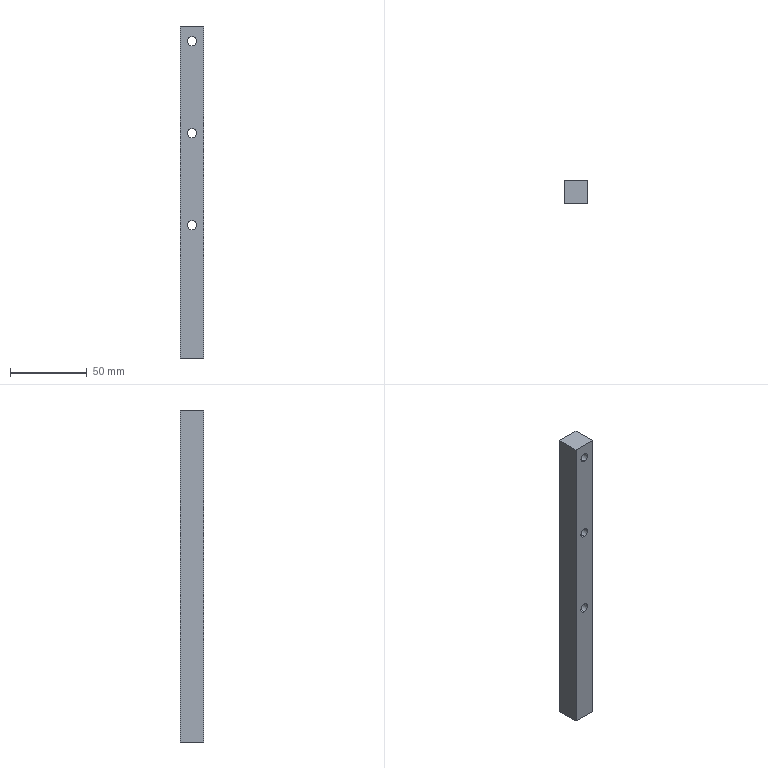Part | 1 solid | 16 faces | box 15 x 15 x 216.5 mm | volume 46834 mm3 | cylinder 8 | plane 6 | cone 2 | commonest cylinder face diameters 6 x6 6.8 x2
STEP:
#1=CARTESIAN_POINT('',(10.9,7.5,59.5));
#2=VERTEX_POINT('',#1);
#3=CARTESIAN_POINT('',(4.1,7.5,59.5));
#4=VERTEX_POINT('',#3);
#5=CARTESIAN_POINT('',(7.5,7.5,59.5));
#6=DIRECTION('',(0.,0.,-1.));
#7=DIRECTION('',(-1.,0.,0.));
#8=AXIS2_PLACEMENT_3D('',#5,#6,#7);
#9=CIRCLE('',#8,3.4);
#10=EDGE_CURVE('',#2,#4,#9,.T.);
#11=ORIENTED_EDGE('',*,*,#10,.F.);
#12=CARTESIAN_POINT('',(10.9,7.5,43.5));
#13=VERTEX_POINT('',#12);
#14=CARTESIAN_POINT('',(10.9,7.5,43.5));
#15=DIRECTION('',(0.,0.,-1.));
#16=VECTOR('',#15,1000.);
#17=LINE('',#14,#16);
#18=EDGE_CURVE('',#2,#13,#17,.T.);
#19=ORIENTED_EDGE('',*,*,#18,.T.);
#20=CARTESIAN_POINT('',(4.1,7.5,43.5));
#21=VERTEX_POINT('',#20);
#22=CARTESIAN_POINT('',(7.5,7.5,43.5));
#23=DIRECTION('',(0.,0.,-1.));
#24=DIRECTION('',(-1.,0.,0.));
#25=AXIS2_PLACEMENT_3D('',#22,#23,#24);
#26=CIRCLE('',#25,3.4);
#27=EDGE_CURVE('',#13,#21,#26,.T.);
#28=ORIENTED_EDGE('',*,*,#27,.T.);
#29=CARTESIAN_POINT('',(4.1,7.5,43.5));
#30=DIRECTION('',(0.,0.,-1.));
#31=VECTOR('',#30,1000.);
#32=LINE('',#29,#31);
#33=EDGE_CURVE('',#4,#21,#32,.T.);
#34=ORIENTED_EDGE('',*,*,#33,.F.);
#35=EDGE_LOOP('',(#11,#19,#28,#34));
#36=FACE_OUTER_BOUND('',#35,.T.);
#37=CARTESIAN_POINT('',(7.5,7.5,43.5));
#38=DIRECTION('',(0.,0.,-1.));
#39=DIRECTION('',(-1.,0.,0.));
#40=AXIS2_PLACEMENT_3D('',#37,#38,#39);
#41=CYLINDRICAL_SURFACE('',#40,3.4);
#42=ADVANCED_FACE('',(#36),#41,.F.);
#43=CARTESIAN_POINT('',(7.5,7.5,61.543));
#44=VERTEX_POINT('',#43);
#45=CARTESIAN_POINT('',(4.1,7.5,59.5));
#46=DIRECTION('',(-0.8572,0.,-0.515));
#47=VECTOR('',#46,1000.);
#48=LINE('',#45,#47);
#49=EDGE_CURVE('',#44,#4,#48,.T.);
#50=ORIENTED_EDGE('',*,*,#49,.F.);
#51=CARTESIAN_POINT('',(10.9,7.5,59.5));
#52=DIRECTION('',(0.8572,0.,-0.515));
#53=VECTOR('',#52,1000.);
#54=LINE('',#51,#53);
#55=EDGE_CURVE('',#44,#2,#54,.T.);
#56=ORIENTED_EDGE('',*,*,#55,.T.);
#57=ORIENTED_EDGE('',*,*,#10,.T.);
#58=EDGE_LOOP('',(#50,#56,#57));
#59=FACE_OUTER_BOUND('',#58,.T.);
#60=CARTESIAN_POINT('',(7.5,7.5,59.5));
#61=DIRECTION('',(0.,0.,-1.));
#62=DIRECTION('',(-1.,0.,0.));
#63=AXIS2_PLACEMENT_3D('',#60,#61,#62);
#64=CONICAL_SURFACE('',#63,3.4,1.03);
#65=ADVANCED_FACE('',(#59),#64,.F.);
#66=CARTESIAN_POINT('',(7.5,0.,247.));
#67=VERTEX_POINT('',#66);
#68=CARTESIAN_POINT('',(7.5,0.,253.));
#69=VERTEX_POINT('',#68);
#70=CARTESIAN_POINT('',(7.5,0.,250.));
#71=DIRECTION('',(0.,1.,0.));
#72=DIRECTION('',(0.,0.,1.));
#73=AXIS2_PLACEMENT_3D('',#70,#71,#72);
#74=CIRCLE('',#73,3.);
#75=EDGE_CURVE('',#67,#69,#74,.T.);
#76=ORIENTED_EDGE('',*,*,#75,.F.);
#77=CARTESIAN_POINT('',(7.5,15.,247.));
#78=VERTEX_POINT('',#77);
#79=CARTESIAN_POINT('',(7.5,-35.,247.));
#80=DIRECTION('',(0.,1.,0.));
#81=VECTOR('',#80,1000.);
#82=LINE('',#79,#81);
#83=EDGE_CURVE('',#67,#78,#82,.T.);
#84=ORIENTED_EDGE('',*,*,#83,.T.);
#85=CARTESIAN_POINT('',(7.5,15.,253.));
#86=VERTEX_POINT('',#85);
#87=CARTESIAN_POINT('',(7.5,15.,250.));
#88=DIRECTION('',(0.,1.,0.));
#89=DIRECTION('',(0.,0.,1.));
#90=AXIS2_PLACEMENT_3D('',#87,#88,#89);
#91=CIRCLE('',#90,3.);
#92=EDGE_CURVE('',#78,#86,#91,.T.);
#93=ORIENTED_EDGE('',*,*,#92,.T.);
#94=CARTESIAN_POINT('',(7.5,-35.,253.));
#95=DIRECTION('',(0.,1.,0.));
#96=VECTOR('',#95,1000.);
#97=LINE('',#94,#96);
#98=EDGE_CURVE('',#69,#86,#97,.T.);
#99=ORIENTED_EDGE('',*,*,#98,.F.);
#100=EDGE_LOOP('',(#76,#84,#93,#99));
#101=FACE_OUTER_BOUND('',#100,.T.);
#102=CARTESIAN_POINT('',(7.5,-35.,250.));
#103=DIRECTION('',(0.,1.,0.));
#104=DIRECTION('',(0.,0.,1.));
#105=AXIS2_PLACEMENT_3D('',#102,#103,#104);
#106=CYLINDRICAL_SURFACE('',#105,3.);
#107=ADVANCED_FACE('',(#101),#106,.F.);
#108=CARTESIAN_POINT('',(7.5,0.,187.));
#109=VERTEX_POINT('',#108);
#110=CARTESIAN_POINT('',(7.5,0.,193.));
#111=VERTEX_POINT('',#110);
#112=CARTESIAN_POINT('',(7.5,0.,190.));
#113=DIRECTION('',(0.,1.,0.));
#114=DIRECTION('',(0.,0.,1.));
#115=AXIS2_PLACEMENT_3D('',#112,#113,#114);
#116=CIRCLE('',#115,3.);
#117=EDGE_CURVE('',#109,#111,#116,.T.);
#118=ORIENTED_EDGE('',*,*,#117,.F.);
#119=CARTESIAN_POINT('',(7.5,15.,187.));
#120=VERTEX_POINT('',#119);
#121=CARTESIAN_POINT('',(7.5,-35.,187.));
#122=DIRECTION('',(0.,1.,0.));
#123=VECTOR('',#122,1000.);
#124=LINE('',#121,#123);
#125=EDGE_CURVE('',#109,#120,#124,.T.);
#126=ORIENTED_EDGE('',*,*,#125,.T.);
#127=CARTESIAN_POINT('',(7.5,15.,193.));
#128=VERTEX_POINT('',#127);
#129=CARTESIAN_POINT('',(7.5,15.,190.));
#130=DIRECTION('',(0.,1.,0.));
#131=DIRECTION('',(0.,0.,1.));
#132=AXIS2_PLACEMENT_3D('',#129,#130,#131);
#133=CIRCLE('',#132,3.);
#134=EDGE_CURVE('',#120,#128,#133,.T.);
#135=ORIENTED_EDGE('',*,*,#134,.T.);
#136=CARTESIAN_POINT('',(7.5,-35.,193.));
#137=DIRECTION('',(0.,1.,0.));
#138=VECTOR('',#137,1000.);
#139=LINE('',#136,#138);
#140=EDGE_CURVE('',#111,#128,#139,.T.);
#141=ORIENTED_EDGE('',*,*,#140,.F.);
#142=EDGE_LOOP('',(#118,#126,#135,#141));
#143=FACE_OUTER_BOUND('',#142,.T.);
#144=CARTESIAN_POINT('',(7.5,-35.,190.));
#145=DIRECTION('',(0.,1.,0.));
#146=DIRECTION('',(0.,0.,1.));
#147=AXIS2_PLACEMENT_3D('',#144,#145,#146);
#148=CYLINDRICAL_SURFACE('',#147,3.);
#149=ADVANCED_FACE('',(#143),#148,.F.);
#150=CARTESIAN_POINT('',(7.5,0.,127.));
#151=VERTEX_POINT('',#150);
#152=CARTESIAN_POINT('',(7.5,0.,133.));
#153=VERTEX_POINT('',#152);
#154=CARTESIAN_POINT('',(7.5,0.,130.));
#155=DIRECTION('',(0.,1.,0.));
#156=DIRECTION('',(0.,0.,1.));
#157=AXIS2_PLACEMENT_3D('',#154,#155,#156);
#158=CIRCLE('',#157,3.);
#159=EDGE_CURVE('',#151,#153,#158,.T.);
#160=ORIENTED_EDGE('',*,*,#159,.F.);
#161=CARTESIAN_POINT('',(7.5,15.,127.));
#162=VERTEX_POINT('',#161);
#163=CARTESIAN_POINT('',(7.5,-35.,127.));
#164=DIRECTION('',(0.,1.,0.));
#165=VECTOR('',#164,1000.);
#166=LINE('',#163,#165);
#167=EDGE_CURVE('',#151,#162,#166,.T.);
#168=ORIENTED_EDGE('',*,*,#167,.T.);
#169=CARTESIAN_POINT('',(7.5,15.,133.));
#170=VERTEX_POINT('',#169);
#171=CARTESIAN_POINT('',(7.5,15.,130.));
#172=DIRECTION('',(0.,1.,0.));
#173=DIRECTION('',(0.,0.,1.));
#174=AXIS2_PLACEMENT_3D('',#171,#172,#173);
#175=CIRCLE('',#174,3.);
#176=EDGE_CURVE('',#162,#170,#175,.T.);
#177=ORIENTED_EDGE('',*,*,#176,.T.);
#178=CARTESIAN_POINT('',(7.5,-35.,133.));
#179=DIRECTION('',(0.,1.,0.));
#180=VECTOR('',#179,1000.);
#181=LINE('',#178,#180);
#182=EDGE_CURVE('',#153,#170,#181,.T.);
#183=ORIENTED_EDGE('',*,*,#182,.F.);
#184=EDGE_LOOP('',(#160,#168,#177,#183));
#185=FACE_OUTER_BOUND('',#184,.T.);
#186=CARTESIAN_POINT('',(7.5,-35.,130.));
#187=DIRECTION('',(0.,1.,0.));
#188=DIRECTION('',(0.,0.,1.));
#189=AXIS2_PLACEMENT_3D('',#186,#187,#188);
#190=CYLINDRICAL_SURFACE('',#189,3.);
#191=ADVANCED_FACE('',(#185),#190,.F.);
#192=CARTESIAN_POINT('',(0.,15.,260.));
#193=VERTEX_POINT('',#192);
#194=CARTESIAN_POINT('',(0.,15.,43.5));
#195=VERTEX_POINT('',#194);
#196=CARTESIAN_POINT('',(0.,15.,700.));
#197=DIRECTION('',(0.,0.,-1.));
#198=VECTOR('',#197,1000.);
#199=LINE('',#196,#198);
#200=EDGE_CURVE('',#193,#195,#199,.T.);
#201=ORIENTED_EDGE('',*,*,#200,.T.);
#202=CARTESIAN_POINT('',(0.,0.,43.5));
#203=VERTEX_POINT('',#202);
#204=CARTESIAN_POINT('',(0.,15.,43.5));
#205=DIRECTION('',(0.,1.,0.));
#206=VECTOR('',#205,1000.);
#207=LINE('',#204,#206);
#208=EDGE_CURVE('',#203,#195,#207,.T.);
#209=ORIENTED_EDGE('',*,*,#208,.F.);
#210=CARTESIAN_POINT('',(0.,0.,260.));
#211=VERTEX_POINT('',#210);
#212=CARTESIAN_POINT('',(0.,0.,700.));
#213=DIRECTION('',(0.,0.,-1.));
#214=VECTOR('',#213,1000.);
#215=LINE('',#212,#214);
#216=EDGE_CURVE('',#211,#203,#215,.T.);
#217=ORIENTED_EDGE('',*,*,#216,.F.);
#218=CARTESIAN_POINT('',(0.,15.,260.));
#219=DIRECTION('',(0.,-1.,0.));
#220=VECTOR('',#219,1000.);
#221=LINE('',#218,#220);
#222=EDGE_CURVE('',#193,#211,#221,.T.);
#223=ORIENTED_EDGE('',*,*,#222,.F.);
#224=EDGE_LOOP('',(#201,#209,#217,#223));
#225=FACE_OUTER_BOUND('',#224,.T.);
#226=CARTESIAN_POINT('',(0.,0.,700.));
#227=DIRECTION('',(1.,0.,0.));
#228=DIRECTION('',(0.,0.,-1.));
#229=AXIS2_PLACEMENT_3D('',#226,#227,#228);
#230=PLANE('',#229);
#231=ADVANCED_FACE('',(#225),#230,.F.);
#232=CARTESIAN_POINT('',(7.5,0.,130.));
#233=DIRECTION('',(0.,1.,0.));
#234=DIRECTION('',(0.,0.,1.));
#235=AXIS2_PLACEMENT_3D('',#232,#233,#234);
#236=CIRCLE('',#235,3.);
#237=EDGE_CURVE('',#153,#151,#236,.T.);
#238=ORIENTED_EDGE('',*,*,#237,.T.);
#239=ORIENTED_EDGE('',*,*,#159,.T.);
#240=EDGE_LOOP('',(#238,#239));
#241=FACE_BOUND('',#240,.T.);
#242=CARTESIAN_POINT('',(7.5,0.,190.));
#243=DIRECTION('',(0.,1.,0.));
#244=DIRECTION('',(0.,0.,1.));
#245=AXIS2_PLACEMENT_3D('',#242,#243,#244);
#246=CIRCLE('',#245,3.);
#247=EDGE_CURVE('',#111,#109,#246,.T.);
#248=ORIENTED_EDGE('',*,*,#247,.T.);
#249=ORIENTED_EDGE('',*,*,#117,.T.);
#250=EDGE_LOOP('',(#248,#249));
#251=FACE_BOUND('',#250,.T.);
#252=CARTESIAN_POINT('',(7.5,0.,250.));
#253=DIRECTION('',(0.,1.,0.));
#254=DIRECTION('',(0.,0.,1.));
#255=AXIS2_PLACEMENT_3D('',#252,#253,#254);
#256=CIRCLE('',#255,3.);
#257=EDGE_CURVE('',#69,#67,#256,.T.);
#258=ORIENTED_EDGE('',*,*,#257,.T.);
#259=ORIENTED_EDGE('',*,*,#75,.T.);
#260=EDGE_LOOP('',(#258,#259));
#261=FACE_BOUND('',#260,.T.);
#262=ORIENTED_EDGE('',*,*,#216,.T.);
#263=CARTESIAN_POINT('',(15.,0.,43.5));
#264=VERTEX_POINT('',#263);
#265=CARTESIAN_POINT('',(15.,0.,43.5));
#266=DIRECTION('',(-1.,0.,0.));
#267=VECTOR('',#266,1000.);
#268=LINE('',#265,#267);
#269=EDGE_CURVE('',#264,#203,#268,.T.);
#270=ORIENTED_EDGE('',*,*,#269,.F.);
#271=CARTESIAN_POINT('',(15.,0.,260.));
#272=VERTEX_POINT('',#271);
#273=CARTESIAN_POINT('',(15.,0.,700.));
#274=DIRECTION('',(0.,0.,-1.));
#275=VECTOR('',#274,1000.);
#276=LINE('',#273,#275);
#277=EDGE_CURVE('',#272,#264,#276,.T.);
#278=ORIENTED_EDGE('',*,*,#277,.F.);
#279=CARTESIAN_POINT('',(0.,0.,260.));
#280=DIRECTION('',(1.,0.,0.));
#281=VECTOR('',#280,1000.);
#282=LINE('',#279,#281);
#283=EDGE_CURVE('',#211,#272,#282,.T.);
#284=ORIENTED_EDGE('',*,*,#283,.F.);
#285=EDGE_LOOP('',(#262,#270,#278,#284));
#286=FACE_OUTER_BOUND('',#285,.T.);
#287=CARTESIAN_POINT('',(0.,0.,700.));
#288=DIRECTION('',(0.,1.,0.));
#289=DIRECTION('',(0.,0.,1.));
#290=AXIS2_PLACEMENT_3D('',#287,#288,#289);
#291=PLANE('',#290);
#292=ADVANCED_FACE('',(#241,#251,#261,#286),#291,.F.);
#293=ORIENTED_EDGE('',*,*,#277,.T.);
#294=CARTESIAN_POINT('',(15.,15.,43.5));
#295=VERTEX_POINT('',#294);
#296=CARTESIAN_POINT('',(15.,15.,43.5));
#297=DIRECTION('',(0.,-1.,0.));
#298=VECTOR('',#297,1000.);
#299=LINE('',#296,#298);
#300=EDGE_CURVE('',#295,#264,#299,.T.);
#301=ORIENTED_EDGE('',*,*,#300,.F.);
#302=CARTESIAN_POINT('',(15.,15.,260.));
#303=VERTEX_POINT('',#302);
#304=CARTESIAN_POINT('',(15.,15.,700.));
#305=DIRECTION('',(0.,0.,-1.));
#306=VECTOR('',#305,1000.);
#307=LINE('',#304,#306);
#308=EDGE_CURVE('',#303,#295,#307,.T.);
#309=ORIENTED_EDGE('',*,*,#308,.F.);
#310=CARTESIAN_POINT('',(15.,0.,260.));
#311=DIRECTION('',(0.,1.,0.));
#312=VECTOR('',#311,1000.);
#313=LINE('',#310,#312);
#314=EDGE_CURVE('',#272,#303,#313,.T.);
#315=ORIENTED_EDGE('',*,*,#314,.F.);
#316=EDGE_LOOP('',(#293,#301,#309,#315));
#317=FACE_OUTER_BOUND('',#316,.T.);
#318=CARTESIAN_POINT('',(15.,0.,700.));
#319=DIRECTION('',(-1.,0.,0.));
#320=DIRECTION('',(0.,0.,1.));
#321=AXIS2_PLACEMENT_3D('',#318,#319,#320);
#322=PLANE('',#321);
#323=ADVANCED_FACE('',(#317),#322,.F.);
#324=CARTESIAN_POINT('',(7.5,15.,130.));
#325=DIRECTION('',(0.,1.,0.));
#326=DIRECTION('',(0.,0.,1.));
#327=AXIS2_PLACEMENT_3D('',#324,#325,#326);
#328=CIRCLE('',#327,3.);
#329=EDGE_CURVE('',#170,#162,#328,.T.);
#330=ORIENTED_EDGE('',*,*,#329,.F.);
#331=ORIENTED_EDGE('',*,*,#176,.F.);
#332=EDGE_LOOP('',(#330,#331));
#333=FACE_BOUND('',#332,.T.);
#334=CARTESIAN_POINT('',(7.5,15.,190.));
#335=DIRECTION('',(0.,1.,0.));
#336=DIRECTION('',(0.,0.,1.));
#337=AXIS2_PLACEMENT_3D('',#334,#335,#336);
#338=CIRCLE('',#337,3.);
#339=EDGE_CURVE('',#128,#120,#338,.T.);
#340=ORIENTED_EDGE('',*,*,#339,.F.);
#341=ORIENTED_EDGE('',*,*,#134,.F.);
#342=EDGE_LOOP('',(#340,#341));
#343=FACE_BOUND('',#342,.T.);
#344=CARTESIAN_POINT('',(7.5,15.,250.));
#345=DIRECTION('',(0.,1.,0.));
#346=DIRECTION('',(0.,0.,1.));
#347=AXIS2_PLACEMENT_3D('',#344,#345,#346);
#348=CIRCLE('',#347,3.);
#349=EDGE_CURVE('',#86,#78,#348,.T.);
#350=ORIENTED_EDGE('',*,*,#349,.F.);
#351=ORIENTED_EDGE('',*,*,#92,.F.);
#352=EDGE_LOOP('',(#350,#351));
#353=FACE_BOUND('',#352,.T.);
#354=ORIENTED_EDGE('',*,*,#308,.T.);
#355=CARTESIAN_POINT('',(15.,15.,43.5));
#356=DIRECTION('',(1.,0.,0.));
#357=VECTOR('',#356,1000.);
#358=LINE('',#355,#357);
#359=EDGE_CURVE('',#195,#295,#358,.T.);
#360=ORIENTED_EDGE('',*,*,#359,.F.);
#361=ORIENTED_EDGE('',*,*,#200,.F.);
#362=CARTESIAN_POINT('',(15.,15.,260.));
#363=DIRECTION('',(-1.,0.,0.));
#364=VECTOR('',#363,1000.);
#365=LINE('',#362,#364);
#366=EDGE_CURVE('',#303,#193,#365,.T.);
#367=ORIENTED_EDGE('',*,*,#366,.F.);
#368=EDGE_LOOP('',(#354,#360,#361,#367));
#369=FACE_OUTER_BOUND('',#368,.T.);
#370=CARTESIAN_POINT('',(0.,15.,700.));
#371=DIRECTION('',(0.,-1.,0.));
#372=DIRECTION('',(0.,0.,-1.));
#373=AXIS2_PLACEMENT_3D('',#370,#371,#372);
#374=PLANE('',#373);
#375=ADVANCED_FACE('',(#333,#343,#353,#369),#374,.F.);
#376=ORIENTED_EDGE('',*,*,#167,.F.);
#377=ORIENTED_EDGE('',*,*,#237,.F.);
#378=ORIENTED_EDGE('',*,*,#182,.T.);
#379=ORIENTED_EDGE('',*,*,#329,.T.);
#380=EDGE_LOOP('',(#376,#377,#378,#379));
#381=FACE_OUTER_BOUND('',#380,.T.);
#382=CARTESIAN_POINT('',(7.5,-35.,130.));
#383=DIRECTION('',(0.,1.,0.));
#384=DIRECTION('',(0.,0.,1.));
#385=AXIS2_PLACEMENT_3D('',#382,#383,#384);
#386=CYLINDRICAL_SURFACE('',#385,3.);
#387=ADVANCED_FACE('',(#381),#386,.F.);
#388=ORIENTED_EDGE('',*,*,#125,.F.);
#389=ORIENTED_EDGE('',*,*,#247,.F.);
#390=ORIENTED_EDGE('',*,*,#140,.T.);
#391=ORIENTED_EDGE('',*,*,#339,.T.);
#392=EDGE_LOOP('',(#388,#389,#390,#391));
#393=FACE_OUTER_BOUND('',#392,.T.);
#394=CARTESIAN_POINT('',(7.5,-35.,190.));
#395=DIRECTION('',(0.,1.,0.));
#396=DIRECTION('',(0.,0.,1.));
#397=AXIS2_PLACEMENT_3D('',#394,#395,#396);
#398=CYLINDRICAL_SURFACE('',#397,3.);
#399=ADVANCED_FACE('',(#393),#398,.F.);
#400=ORIENTED_EDGE('',*,*,#83,.F.);
#401=ORIENTED_EDGE('',*,*,#257,.F.);
#402=ORIENTED_EDGE('',*,*,#98,.T.);
#403=ORIENTED_EDGE('',*,*,#349,.T.);
#404=EDGE_LOOP('',(#400,#401,#402,#403));
#405=FACE_OUTER_BOUND('',#404,.T.);
#406=CARTESIAN_POINT('',(7.5,-35.,250.));
#407=DIRECTION('',(0.,1.,0.));
#408=DIRECTION('',(0.,0.,1.));
#409=AXIS2_PLACEMENT_3D('',#406,#407,#408);
#410=CYLINDRICAL_SURFACE('',#409,3.);
#411=ADVANCED_FACE('',(#405),#410,.F.);
#412=ORIENTED_EDGE('',*,*,#366,.T.);
#413=ORIENTED_EDGE('',*,*,#222,.T.);
#414=ORIENTED_EDGE('',*,*,#283,.T.);
#415=ORIENTED_EDGE('',*,*,#314,.T.);
#416=EDGE_LOOP('',(#412,#413,#414,#415));
#417=FACE_OUTER_BOUND('',#416,.T.);
#418=CARTESIAN_POINT('',(0.,0.,260.));
#419=DIRECTION('',(0.,0.,1.));
#420=DIRECTION('',(1.,0.,0.));
#421=AXIS2_PLACEMENT_3D('',#418,#419,#420);
#422=PLANE('',#421);
#423=ADVANCED_FACE('',(#417),#422,.T.);
#424=CARTESIAN_POINT('',(7.5,7.5,43.5));
#425=DIRECTION('',(0.,0.,-1.));
#426=DIRECTION('',(-1.,0.,0.));
#427=AXIS2_PLACEMENT_3D('',#424,#425,#426);
#428=CIRCLE('',#427,3.4);
#429=EDGE_CURVE('',#21,#13,#428,.T.);
#430=ORIENTED_EDGE('',*,*,#429,.F.);
#431=ORIENTED_EDGE('',*,*,#27,.F.);
#432=EDGE_LOOP('',(#430,#431));
#433=FACE_BOUND('',#432,.T.);
#434=ORIENTED_EDGE('',*,*,#300,.T.);
#435=ORIENTED_EDGE('',*,*,#269,.T.);
#436=ORIENTED_EDGE('',*,*,#208,.T.);
#437=ORIENTED_EDGE('',*,*,#359,.T.);
#438=EDGE_LOOP('',(#434,#435,#436,#437));
#439=FACE_OUTER_BOUND('',#438,.T.);
#440=CARTESIAN_POINT('',(0.,0.,43.5));
#441=DIRECTION('',(0.,0.,-1.));
#442=DIRECTION('',(-1.,0.,0.));
#443=AXIS2_PLACEMENT_3D('',#440,#441,#442);
#444=PLANE('',#443);
#445=ADVANCED_FACE('',(#433,#439),#444,.T.);
#446=ORIENTED_EDGE('',*,*,#55,.F.);
#447=ORIENTED_EDGE('',*,*,#49,.T.);
#448=CARTESIAN_POINT('',(7.5,7.5,59.5));
#449=DIRECTION('',(0.,0.,-1.));
#450=DIRECTION('',(-1.,0.,0.));
#451=AXIS2_PLACEMENT_3D('',#448,#449,#450);
#452=CIRCLE('',#451,3.4);
#453=EDGE_CURVE('',#4,#2,#452,.T.);
#454=ORIENTED_EDGE('',*,*,#453,.T.);
#455=EDGE_LOOP('',(#446,#447,#454));
#456=FACE_OUTER_BOUND('',#455,.T.);
#457=CARTESIAN_POINT('',(7.5,7.5,59.5));
#458=DIRECTION('',(0.,0.,-1.));
#459=DIRECTION('',(-1.,0.,0.));
#460=AXIS2_PLACEMENT_3D('',#457,#458,#459);
#461=CONICAL_SURFACE('',#460,3.4,1.03);
#462=ADVANCED_FACE('',(#456),#461,.F.);
#463=ORIENTED_EDGE('',*,*,#18,.F.);
#464=ORIENTED_EDGE('',*,*,#453,.F.);
#465=ORIENTED_EDGE('',*,*,#33,.T.);
#466=ORIENTED_EDGE('',*,*,#429,.T.);
#467=EDGE_LOOP('',(#463,#464,#465,#466));
#468=FACE_OUTER_BOUND('',#467,.T.);
#469=CARTESIAN_POINT('',(7.5,7.5,43.5));
#470=DIRECTION('',(0.,0.,-1.));
#471=DIRECTION('',(-1.,0.,0.));
#472=AXIS2_PLACEMENT_3D('',#469,#470,#471);
#473=CYLINDRICAL_SURFACE('',#472,3.4);
#474=ADVANCED_FACE('',(#468),#473,.F.);
#475=CLOSED_SHELL('',(#42,#65,#107,#149,#191,#231,#292,#323,#375,#387,#399,#411,#423,#445,#462,#474));
#476=MANIFOLD_SOLID_BREP('',#475);
#477=CARTESIAN_POINT('',(0.,0.,0.));
#478=DIRECTION('',(0.,0.,1.));
#479=DIRECTION('',(1.,0.,0.));
#480=AXIS2_PLACEMENT_3D('',#477,#478,#479);
#481=(LENGTH_UNIT()NAMED_UNIT(*)SI_UNIT(.MILLI.,.METRE.));
#482=UNCERTAINTY_MEASURE_WITH_UNIT(LENGTH_MEASURE(0.00001),#481,'','');
#483=(NAMED_UNIT(*)PLANE_ANGLE_UNIT()SI_UNIT($,.RADIAN.));
#484=(NAMED_UNIT(*)SI_UNIT($,.STERADIAN.)SOLID_ANGLE_UNIT());
#485=(GEOMETRIC_REPRESENTATION_CONTEXT(3)GLOBAL_UNCERTAINTY_ASSIGNED_CONTEXT((#482))GLOBAL_UNIT_ASSIGNED_CONTEXT((#481,#483,#484))REPRESENTATION_CONTEXT('',''));
#486=ADVANCED_BREP_SHAPE_REPRESENTATION('',(#476,#480),#485);